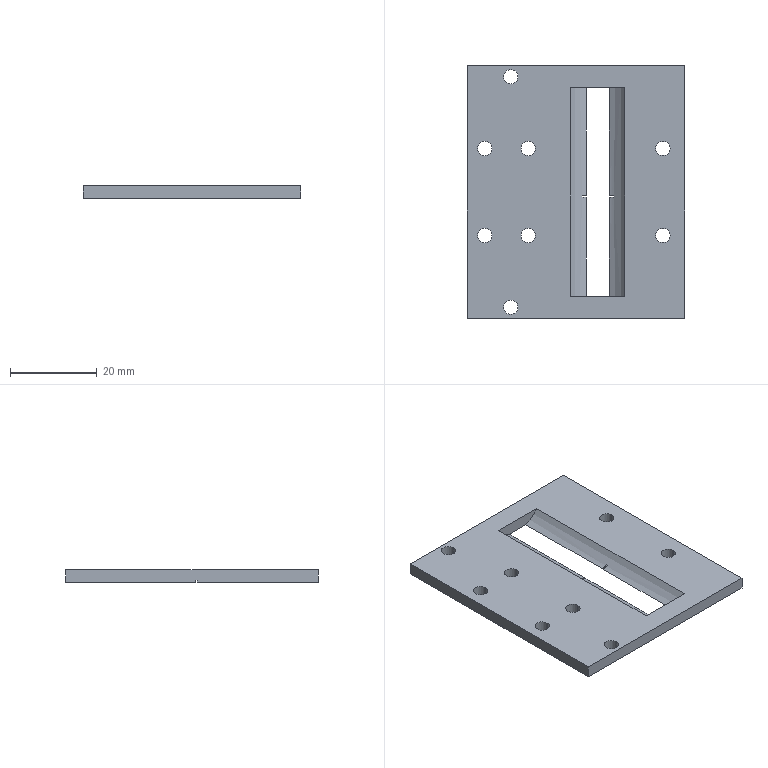Part | SolidWorks | features ICE 3, Extrusion 1 | 1 solid | 33 faces | box 50 x 58 x 2.8 mm | volume 6623 mm3 | cylinder 18 | plane 15 | commonest cylinder face diameters 3.3 x16 15 x2
STEP:
#1=CARTESIAN_POINT('',(-30.658,18.937,0.));
#2=VERTEX_POINT('',#1);
#3=CARTESIAN_POINT('',(-27.358,18.937,0.));
#4=VERTEX_POINT('',#3);
#5=CARTESIAN_POINT('',(-29.008,18.937,0.));
#6=DIRECTION('',(0.,0.,1.));
#7=DIRECTION('',(1.,0.,0.));
#8=AXIS2_PLACEMENT_3D('',#5,#6,#7);
#9=CIRCLE('',#8,1.65);
#10=EDGE_CURVE('',#2,#4,#9,.T.);
#11=ORIENTED_EDGE('',*,*,#10,.F.);
#12=CARTESIAN_POINT('',(-30.658,18.937,2.8));
#13=VERTEX_POINT('',#12);
#14=CARTESIAN_POINT('',(-30.658,18.937,0.));
#15=DIRECTION('',(0.,0.,1.));
#16=VECTOR('',#15,1000.);
#17=LINE('',#14,#16);
#18=EDGE_CURVE('',#2,#13,#17,.T.);
#19=ORIENTED_EDGE('',*,*,#18,.T.);
#20=CARTESIAN_POINT('',(-27.358,18.937,2.8));
#21=VERTEX_POINT('',#20);
#22=CARTESIAN_POINT('',(-29.008,18.937,2.8));
#23=DIRECTION('',(0.,0.,1.));
#24=DIRECTION('',(1.,0.,0.));
#25=AXIS2_PLACEMENT_3D('',#22,#23,#24);
#26=CIRCLE('',#25,1.65);
#27=EDGE_CURVE('',#13,#21,#26,.T.);
#28=ORIENTED_EDGE('',*,*,#27,.T.);
#29=CARTESIAN_POINT('',(-27.358,18.937,0.));
#30=DIRECTION('',(0.,0.,1.));
#31=VECTOR('',#30,1000.);
#32=LINE('',#29,#31);
#33=EDGE_CURVE('',#4,#21,#32,.T.);
#34=ORIENTED_EDGE('',*,*,#33,.F.);
#35=EDGE_LOOP('',(#11,#19,#28,#34));
#36=FACE_OUTER_BOUND('',#35,.T.);
#37=CARTESIAN_POINT('',(-29.008,18.937,0.));
#38=DIRECTION('',(0.,0.,1.));
#39=DIRECTION('',(1.,0.,0.));
#40=AXIS2_PLACEMENT_3D('',#37,#38,#39);
#41=CYLINDRICAL_SURFACE('',#40,1.65);
#42=ADVANCED_FACE('',(#36),#41,.F.);
#43=CARTESIAN_POINT('',(4.342,-17.563,0.));
#44=VERTEX_POINT('',#43);
#45=CARTESIAN_POINT('',(7.642,-17.563,0.));
#46=VERTEX_POINT('',#45);
#47=CARTESIAN_POINT('',(5.992,-17.563,0.));
#48=DIRECTION('',(0.,0.,1.));
#49=DIRECTION('',(1.,0.,0.));
#50=AXIS2_PLACEMENT_3D('',#47,#48,#49);
#51=CIRCLE('',#50,1.65);
#52=EDGE_CURVE('',#44,#46,#51,.T.);
#53=ORIENTED_EDGE('',*,*,#52,.F.);
#54=CARTESIAN_POINT('',(4.342,-17.563,2.8));
#55=VERTEX_POINT('',#54);
#56=CARTESIAN_POINT('',(4.342,-17.563,0.));
#57=DIRECTION('',(0.,0.,1.));
#58=VECTOR('',#57,1000.);
#59=LINE('',#56,#58);
#60=EDGE_CURVE('',#44,#55,#59,.T.);
#61=ORIENTED_EDGE('',*,*,#60,.T.);
#62=CARTESIAN_POINT('',(7.642,-17.563,2.8));
#63=VERTEX_POINT('',#62);
#64=CARTESIAN_POINT('',(5.992,-17.563,2.8));
#65=DIRECTION('',(0.,0.,1.));
#66=DIRECTION('',(1.,0.,0.));
#67=AXIS2_PLACEMENT_3D('',#64,#65,#66);
#68=CIRCLE('',#67,1.65);
#69=EDGE_CURVE('',#55,#63,#68,.T.);
#70=ORIENTED_EDGE('',*,*,#69,.T.);
#71=CARTESIAN_POINT('',(7.642,-17.563,0.));
#72=DIRECTION('',(0.,0.,1.));
#73=VECTOR('',#72,1000.);
#74=LINE('',#71,#73);
#75=EDGE_CURVE('',#46,#63,#74,.T.);
#76=ORIENTED_EDGE('',*,*,#75,.F.);
#77=EDGE_LOOP('',(#53,#61,#70,#76));
#78=FACE_OUTER_BOUND('',#77,.T.);
#79=CARTESIAN_POINT('',(5.992,-17.563,0.));
#80=DIRECTION('',(0.,0.,1.));
#81=DIRECTION('',(1.,0.,0.));
#82=AXIS2_PLACEMENT_3D('',#79,#80,#81);
#83=CYLINDRICAL_SURFACE('',#82,1.65);
#84=ADVANCED_FACE('',(#78),#83,.F.);
#85=CARTESIAN_POINT('',(-30.658,-34.063,0.));
#86=VERTEX_POINT('',#85);
#87=CARTESIAN_POINT('',(-27.358,-34.063,0.));
#88=VERTEX_POINT('',#87);
#89=CARTESIAN_POINT('',(-29.008,-34.063,0.));
#90=DIRECTION('',(0.,0.,1.));
#91=DIRECTION('',(1.,0.,0.));
#92=AXIS2_PLACEMENT_3D('',#89,#90,#91);
#93=CIRCLE('',#92,1.65);
#94=EDGE_CURVE('',#86,#88,#93,.T.);
#95=ORIENTED_EDGE('',*,*,#94,.F.);
#96=CARTESIAN_POINT('',(-30.658,-34.063,2.8));
#97=VERTEX_POINT('',#96);
#98=CARTESIAN_POINT('',(-30.658,-34.063,0.));
#99=DIRECTION('',(0.,0.,1.));
#100=VECTOR('',#99,1000.);
#101=LINE('',#98,#100);
#102=EDGE_CURVE('',#86,#97,#101,.T.);
#103=ORIENTED_EDGE('',*,*,#102,.T.);
#104=CARTESIAN_POINT('',(-27.358,-34.063,2.8));
#105=VERTEX_POINT('',#104);
#106=CARTESIAN_POINT('',(-29.008,-34.063,2.8));
#107=DIRECTION('',(0.,0.,1.));
#108=DIRECTION('',(1.,0.,0.));
#109=AXIS2_PLACEMENT_3D('',#106,#107,#108);
#110=CIRCLE('',#109,1.65);
#111=EDGE_CURVE('',#97,#105,#110,.T.);
#112=ORIENTED_EDGE('',*,*,#111,.T.);
#113=CARTESIAN_POINT('',(-27.358,-34.063,0.));
#114=DIRECTION('',(0.,0.,1.));
#115=VECTOR('',#114,1000.);
#116=LINE('',#113,#115);
#117=EDGE_CURVE('',#88,#105,#116,.T.);
#118=ORIENTED_EDGE('',*,*,#117,.F.);
#119=EDGE_LOOP('',(#95,#103,#112,#118));
#120=FACE_OUTER_BOUND('',#119,.T.);
#121=CARTESIAN_POINT('',(-29.008,-34.063,0.));
#122=DIRECTION('',(0.,0.,1.));
#123=DIRECTION('',(1.,0.,0.));
#124=AXIS2_PLACEMENT_3D('',#121,#122,#123);
#125=CYLINDRICAL_SURFACE('',#124,1.65);
#126=ADVANCED_FACE('',(#120),#125,.F.);
#127=CARTESIAN_POINT('',(-26.658,-17.563,0.));
#128=VERTEX_POINT('',#127);
#129=CARTESIAN_POINT('',(-23.358,-17.563,0.));
#130=VERTEX_POINT('',#129);
#131=CARTESIAN_POINT('',(-25.008,-17.563,0.));
#132=DIRECTION('',(0.,0.,1.));
#133=DIRECTION('',(1.,0.,0.));
#134=AXIS2_PLACEMENT_3D('',#131,#132,#133);
#135=CIRCLE('',#134,1.65);
#136=EDGE_CURVE('',#128,#130,#135,.T.);
#137=ORIENTED_EDGE('',*,*,#136,.F.);
#138=CARTESIAN_POINT('',(-26.658,-17.563,2.8));
#139=VERTEX_POINT('',#138);
#140=CARTESIAN_POINT('',(-26.658,-17.563,0.));
#141=DIRECTION('',(0.,0.,1.));
#142=VECTOR('',#141,1000.);
#143=LINE('',#140,#142);
#144=EDGE_CURVE('',#128,#139,#143,.T.);
#145=ORIENTED_EDGE('',*,*,#144,.T.);
#146=CARTESIAN_POINT('',(-23.358,-17.563,2.8));
#147=VERTEX_POINT('',#146);
#148=CARTESIAN_POINT('',(-25.008,-17.563,2.8));
#149=DIRECTION('',(0.,0.,1.));
#150=DIRECTION('',(1.,0.,0.));
#151=AXIS2_PLACEMENT_3D('',#148,#149,#150);
#152=CIRCLE('',#151,1.65);
#153=EDGE_CURVE('',#139,#147,#152,.T.);
#154=ORIENTED_EDGE('',*,*,#153,.T.);
#155=CARTESIAN_POINT('',(-23.358,-17.563,0.));
#156=DIRECTION('',(0.,0.,1.));
#157=VECTOR('',#156,1000.);
#158=LINE('',#155,#157);
#159=EDGE_CURVE('',#130,#147,#158,.T.);
#160=ORIENTED_EDGE('',*,*,#159,.F.);
#161=EDGE_LOOP('',(#137,#145,#154,#160));
#162=FACE_OUTER_BOUND('',#161,.T.);
#163=CARTESIAN_POINT('',(-25.008,-17.563,0.));
#164=DIRECTION('',(0.,0.,1.));
#165=DIRECTION('',(1.,0.,0.));
#166=AXIS2_PLACEMENT_3D('',#163,#164,#165);
#167=CYLINDRICAL_SURFACE('',#166,1.65);
#168=ADVANCED_FACE('',(#162),#167,.F.);
#169=CARTESIAN_POINT('',(-36.658,2.437,0.));
#170=VERTEX_POINT('',#169);
#171=CARTESIAN_POINT('',(-33.358,2.437,0.));
#172=VERTEX_POINT('',#171);
#173=CARTESIAN_POINT('',(-35.008,2.437,0.));
#174=DIRECTION('',(0.,0.,1.));
#175=DIRECTION('',(1.,0.,0.));
#176=AXIS2_PLACEMENT_3D('',#173,#174,#175);
#177=CIRCLE('',#176,1.65);
#178=EDGE_CURVE('',#170,#172,#177,.T.);
#179=ORIENTED_EDGE('',*,*,#178,.F.);
#180=CARTESIAN_POINT('',(-36.658,2.437,2.8));
#181=VERTEX_POINT('',#180);
#182=CARTESIAN_POINT('',(-36.658,2.437,0.));
#183=DIRECTION('',(0.,0.,1.));
#184=VECTOR('',#183,1000.);
#185=LINE('',#182,#184);
#186=EDGE_CURVE('',#170,#181,#185,.T.);
#187=ORIENTED_EDGE('',*,*,#186,.T.);
#188=CARTESIAN_POINT('',(-33.358,2.437,2.8));
#189=VERTEX_POINT('',#188);
#190=CARTESIAN_POINT('',(-35.008,2.437,2.8));
#191=DIRECTION('',(0.,0.,1.));
#192=DIRECTION('',(1.,0.,0.));
#193=AXIS2_PLACEMENT_3D('',#190,#191,#192);
#194=CIRCLE('',#193,1.65);
#195=EDGE_CURVE('',#181,#189,#194,.T.);
#196=ORIENTED_EDGE('',*,*,#195,.T.);
#197=CARTESIAN_POINT('',(-33.358,2.437,0.));
#198=DIRECTION('',(0.,0.,1.));
#199=VECTOR('',#198,1000.);
#200=LINE('',#197,#199);
#201=EDGE_CURVE('',#172,#189,#200,.T.);
#202=ORIENTED_EDGE('',*,*,#201,.F.);
#203=EDGE_LOOP('',(#179,#187,#196,#202));
#204=FACE_OUTER_BOUND('',#203,.T.);
#205=CARTESIAN_POINT('',(-35.008,2.437,0.));
#206=DIRECTION('',(0.,0.,1.));
#207=DIRECTION('',(1.,0.,0.));
#208=AXIS2_PLACEMENT_3D('',#205,#206,#207);
#209=CYLINDRICAL_SURFACE('',#208,1.65);
#210=ADVANCED_FACE('',(#204),#209,.F.);
#211=CARTESIAN_POINT('',(-26.658,2.437,0.));
#212=VERTEX_POINT('',#211);
#213=CARTESIAN_POINT('',(-23.358,2.437,0.));
#214=VERTEX_POINT('',#213);
#215=CARTESIAN_POINT('',(-25.008,2.437,0.));
#216=DIRECTION('',(0.,0.,1.));
#217=DIRECTION('',(1.,0.,0.));
#218=AXIS2_PLACEMENT_3D('',#215,#216,#217);
#219=CIRCLE('',#218,1.65);
#220=EDGE_CURVE('',#212,#214,#219,.T.);
#221=ORIENTED_EDGE('',*,*,#220,.F.);
#222=CARTESIAN_POINT('',(-26.658,2.437,2.8));
#223=VERTEX_POINT('',#222);
#224=CARTESIAN_POINT('',(-26.658,2.437,0.));
#225=DIRECTION('',(0.,0.,1.));
#226=VECTOR('',#225,1000.);
#227=LINE('',#224,#226);
#228=EDGE_CURVE('',#212,#223,#227,.T.);
#229=ORIENTED_EDGE('',*,*,#228,.T.);
#230=CARTESIAN_POINT('',(-23.358,2.437,2.8));
#231=VERTEX_POINT('',#230);
#232=CARTESIAN_POINT('',(-25.008,2.437,2.8));
#233=DIRECTION('',(0.,0.,1.));
#234=DIRECTION('',(1.,0.,0.));
#235=AXIS2_PLACEMENT_3D('',#232,#233,#234);
#236=CIRCLE('',#235,1.65);
#237=EDGE_CURVE('',#223,#231,#236,.T.);
#238=ORIENTED_EDGE('',*,*,#237,.T.);
#239=CARTESIAN_POINT('',(-23.358,2.437,0.));
#240=DIRECTION('',(0.,0.,1.));
#241=VECTOR('',#240,1000.);
#242=LINE('',#239,#241);
#243=EDGE_CURVE('',#214,#231,#242,.T.);
#244=ORIENTED_EDGE('',*,*,#243,.F.);
#245=EDGE_LOOP('',(#221,#229,#238,#244));
#246=FACE_OUTER_BOUND('',#245,.T.);
#247=CARTESIAN_POINT('',(-25.008,2.437,0.));
#248=DIRECTION('',(0.,0.,1.));
#249=DIRECTION('',(1.,0.,0.));
#250=AXIS2_PLACEMENT_3D('',#247,#248,#249);
#251=CYLINDRICAL_SURFACE('',#250,1.65);
#252=ADVANCED_FACE('',(#246),#251,.F.);
#253=CARTESIAN_POINT('',(4.342,2.437,0.));
#254=VERTEX_POINT('',#253);
#255=CARTESIAN_POINT('',(7.642,2.437,0.));
#256=VERTEX_POINT('',#255);
#257=CARTESIAN_POINT('',(5.992,2.437,0.));
#258=DIRECTION('',(0.,0.,1.));
#259=DIRECTION('',(1.,0.,0.));
#260=AXIS2_PLACEMENT_3D('',#257,#258,#259);
#261=CIRCLE('',#260,1.65);
#262=EDGE_CURVE('',#254,#256,#261,.T.);
#263=ORIENTED_EDGE('',*,*,#262,.F.);
#264=CARTESIAN_POINT('',(4.342,2.437,2.8));
#265=VERTEX_POINT('',#264);
#266=CARTESIAN_POINT('',(4.342,2.437,0.));
#267=DIRECTION('',(0.,0.,1.));
#268=VECTOR('',#267,1000.);
#269=LINE('',#266,#268);
#270=EDGE_CURVE('',#254,#265,#269,.T.);
#271=ORIENTED_EDGE('',*,*,#270,.T.);
#272=CARTESIAN_POINT('',(7.642,2.437,2.8));
#273=VERTEX_POINT('',#272);
#274=CARTESIAN_POINT('',(5.992,2.437,2.8));
#275=DIRECTION('',(0.,0.,1.));
#276=DIRECTION('',(1.,0.,0.));
#277=AXIS2_PLACEMENT_3D('',#274,#275,#276);
#278=CIRCLE('',#277,1.65);
#279=EDGE_CURVE('',#265,#273,#278,.T.);
#280=ORIENTED_EDGE('',*,*,#279,.T.);
#281=CARTESIAN_POINT('',(7.642,2.437,0.));
#282=DIRECTION('',(0.,0.,1.));
#283=VECTOR('',#282,1000.);
#284=LINE('',#281,#283);
#285=EDGE_CURVE('',#256,#273,#284,.T.);
#286=ORIENTED_EDGE('',*,*,#285,.F.);
#287=EDGE_LOOP('',(#263,#271,#280,#286));
#288=FACE_OUTER_BOUND('',#287,.T.);
#289=CARTESIAN_POINT('',(5.992,2.437,0.));
#290=DIRECTION('',(0.,0.,1.));
#291=DIRECTION('',(1.,0.,0.));
#292=AXIS2_PLACEMENT_3D('',#289,#290,#291);
#293=CYLINDRICAL_SURFACE('',#292,1.65);
#294=ADVANCED_FACE('',(#288),#293,.F.);
#295=CARTESIAN_POINT('',(-36.658,-17.563,0.));
#296=VERTEX_POINT('',#295);
#297=CARTESIAN_POINT('',(-33.358,-17.563,0.));
#298=VERTEX_POINT('',#297);
#299=CARTESIAN_POINT('',(-35.008,-17.563,0.));
#300=DIRECTION('',(0.,0.,1.));
#301=DIRECTION('',(1.,0.,0.));
#302=AXIS2_PLACEMENT_3D('',#299,#300,#301);
#303=CIRCLE('',#302,1.65);
#304=EDGE_CURVE('',#296,#298,#303,.T.);
#305=ORIENTED_EDGE('',*,*,#304,.F.);
#306=CARTESIAN_POINT('',(-36.658,-17.563,2.8));
#307=VERTEX_POINT('',#306);
#308=CARTESIAN_POINT('',(-36.658,-17.563,0.));
#309=DIRECTION('',(0.,0.,1.));
#310=VECTOR('',#309,1000.);
#311=LINE('',#308,#310);
#312=EDGE_CURVE('',#296,#307,#311,.T.);
#313=ORIENTED_EDGE('',*,*,#312,.T.);
#314=CARTESIAN_POINT('',(-33.358,-17.563,2.8));
#315=VERTEX_POINT('',#314);
#316=CARTESIAN_POINT('',(-35.008,-17.563,2.8));
#317=DIRECTION('',(0.,0.,1.));
#318=DIRECTION('',(1.,0.,0.));
#319=AXIS2_PLACEMENT_3D('',#316,#317,#318);
#320=CIRCLE('',#319,1.65);
#321=EDGE_CURVE('',#307,#315,#320,.T.);
#322=ORIENTED_EDGE('',*,*,#321,.T.);
#323=CARTESIAN_POINT('',(-33.358,-17.563,0.));
#324=DIRECTION('',(0.,0.,1.));
#325=VECTOR('',#324,1000.);
#326=LINE('',#323,#325);
#327=EDGE_CURVE('',#298,#315,#326,.T.);
#328=ORIENTED_EDGE('',*,*,#327,.F.);
#329=EDGE_LOOP('',(#305,#313,#322,#328));
#330=FACE_OUTER_BOUND('',#329,.T.);
#331=CARTESIAN_POINT('',(-35.008,-17.563,0.));
#332=DIRECTION('',(0.,0.,1.));
#333=DIRECTION('',(1.,0.,0.));
#334=AXIS2_PLACEMENT_3D('',#331,#332,#333);
#335=CYLINDRICAL_SURFACE('',#334,1.65);
#336=ADVANCED_FACE('',(#330),#335,.F.);
#337=CARTESIAN_POINT('',(-29.008,18.937,2.8));
#338=DIRECTION('',(0.,0.,1.));
#339=DIRECTION('',(1.,0.,0.));
#340=AXIS2_PLACEMENT_3D('',#337,#338,#339);
#341=CIRCLE('',#340,1.65);
#342=EDGE_CURVE('',#21,#13,#341,.T.);
#343=ORIENTED_EDGE('',*,*,#342,.F.);
#344=ORIENTED_EDGE('',*,*,#27,.F.);
#345=EDGE_LOOP('',(#343,#344));
#346=FACE_BOUND('',#345,.T.);
#347=CARTESIAN_POINT('',(5.992,-17.563,2.8));
#348=DIRECTION('',(0.,0.,1.));
#349=DIRECTION('',(1.,0.,0.));
#350=AXIS2_PLACEMENT_3D('',#347,#348,#349);
#351=CIRCLE('',#350,1.65);
#352=EDGE_CURVE('',#63,#55,#351,.T.);
#353=ORIENTED_EDGE('',*,*,#352,.F.);
#354=ORIENTED_EDGE('',*,*,#69,.F.);
#355=EDGE_LOOP('',(#353,#354));
#356=FACE_BOUND('',#355,.T.);
#357=CARTESIAN_POINT('',(-29.008,-34.063,2.8));
#358=DIRECTION('',(0.,0.,1.));
#359=DIRECTION('',(1.,0.,0.));
#360=AXIS2_PLACEMENT_3D('',#357,#358,#359);
#361=CIRCLE('',#360,1.65);
#362=EDGE_CURVE('',#105,#97,#361,.T.);
#363=ORIENTED_EDGE('',*,*,#362,.F.);
#364=ORIENTED_EDGE('',*,*,#111,.F.);
#365=EDGE_LOOP('',(#363,#364));
#366=FACE_BOUND('',#365,.T.);
#367=CARTESIAN_POINT('',(-25.008,-17.563,2.8));
#368=DIRECTION('',(0.,0.,1.));
#369=DIRECTION('',(1.,0.,0.));
#370=AXIS2_PLACEMENT_3D('',#367,#368,#369);
#371=CIRCLE('',#370,1.65);
#372=EDGE_CURVE('',#147,#139,#371,.T.);
#373=ORIENTED_EDGE('',*,*,#372,.F.);
#374=ORIENTED_EDGE('',*,*,#153,.F.);
#375=EDGE_LOOP('',(#373,#374));
#376=FACE_BOUND('',#375,.T.);
#377=CARTESIAN_POINT('',(-35.008,2.437,2.8));
#378=DIRECTION('',(0.,0.,1.));
#379=DIRECTION('',(1.,0.,0.));
#380=AXIS2_PLACEMENT_3D('',#377,#378,#379);
#381=CIRCLE('',#380,1.65);
#382=EDGE_CURVE('',#189,#181,#381,.T.);
#383=ORIENTED_EDGE('',*,*,#382,.F.);
#384=ORIENTED_EDGE('',*,*,#195,.F.);
#385=EDGE_LOOP('',(#383,#384));
#386=FACE_BOUND('',#385,.T.);
#387=CARTESIAN_POINT('',(-25.008,2.437,2.8));
#388=DIRECTION('',(0.,0.,1.));
#389=DIRECTION('',(1.,0.,0.));
#390=AXIS2_PLACEMENT_3D('',#387,#388,#389);
#391=CIRCLE('',#390,1.65);
#392=EDGE_CURVE('',#231,#223,#391,.T.);
#393=ORIENTED_EDGE('',*,*,#392,.F.);
#394=ORIENTED_EDGE('',*,*,#237,.F.);
#395=EDGE_LOOP('',(#393,#394));
#396=FACE_BOUND('',#395,.T.);
#397=CARTESIAN_POINT('',(5.992,2.437,2.8));
#398=DIRECTION('',(0.,0.,1.));
#399=DIRECTION('',(1.,0.,0.));
#400=AXIS2_PLACEMENT_3D('',#397,#398,#399);
#401=CIRCLE('',#400,1.65);
#402=EDGE_CURVE('',#273,#265,#401,.T.);
#403=ORIENTED_EDGE('',*,*,#402,.F.);
#404=ORIENTED_EDGE('',*,*,#279,.F.);
#405=EDGE_LOOP('',(#403,#404));
#406=FACE_BOUND('',#405,.T.);
#407=CARTESIAN_POINT('',(-35.008,-17.563,2.8));
#408=DIRECTION('',(0.,0.,1.));
#409=DIRECTION('',(1.,0.,0.));
#410=AXIS2_PLACEMENT_3D('',#407,#408,#409);
#411=CIRCLE('',#410,1.65);
#412=EDGE_CURVE('',#315,#307,#411,.T.);
#413=ORIENTED_EDGE('',*,*,#412,.F.);
#414=ORIENTED_EDGE('',*,*,#321,.F.);
#415=EDGE_LOOP('',(#413,#414));
#416=FACE_BOUND('',#415,.T.);
#417=CARTESIAN_POINT('',(-39.008,21.437,2.8));
#418=VERTEX_POINT('',#417);
#419=CARTESIAN_POINT('',(-39.008,-36.563,2.8));
#420=VERTEX_POINT('',#419);
#421=CARTESIAN_POINT('',(-39.008,21.437,2.8));
#422=DIRECTION('',(0.,-1.,0.));
#423=VECTOR('',#422,1000.);
#424=LINE('',#421,#423);
#425=EDGE_CURVE('',#418,#420,#424,.T.);
#426=ORIENTED_EDGE('',*,*,#425,.T.);
#427=CARTESIAN_POINT('',(10.992,-36.563,2.8));
#428=VERTEX_POINT('',#427);
#429=CARTESIAN_POINT('',(-39.008,-36.563,2.8));
#430=DIRECTION('',(1.,0.,0.));
#431=VECTOR('',#430,1000.);
#432=LINE('',#429,#431);
#433=EDGE_CURVE('',#420,#428,#432,.T.);
#434=ORIENTED_EDGE('',*,*,#433,.T.);
#435=CARTESIAN_POINT('',(10.992,21.437,2.8));
#436=VERTEX_POINT('',#435);
#437=CARTESIAN_POINT('',(10.992,21.437,2.8));
#438=DIRECTION('',(0.,1.,0.));
#439=VECTOR('',#438,1000.);
#440=LINE('',#437,#439);
#441=EDGE_CURVE('',#428,#436,#440,.T.);
#442=ORIENTED_EDGE('',*,*,#441,.T.);
#443=CARTESIAN_POINT('',(-39.008,21.437,2.8));
#444=DIRECTION('',(-1.,0.,0.));
#445=VECTOR('',#444,1000.);
#446=LINE('',#443,#445);
#447=EDGE_CURVE('',#436,#418,#446,.T.);
#448=ORIENTED_EDGE('',*,*,#447,.T.);
#449=EDGE_LOOP('',(#426,#434,#442,#448));
#450=FACE_OUTER_BOUND('',#449,.T.);
#451=CARTESIAN_POINT('',(-2.794,-31.563,2.8));
#452=VERTEX_POINT('',#451);
#453=CARTESIAN_POINT('',(-2.794,16.437,2.8));
#454=VERTEX_POINT('',#453);
#455=CARTESIAN_POINT('',(-2.794,-31.563,2.8));
#456=DIRECTION('',(0.,1.,0.));
#457=VECTOR('',#456,1000.);
#458=LINE('',#455,#457);
#459=EDGE_CURVE('',#452,#454,#458,.T.);
#460=ORIENTED_EDGE('',*,*,#459,.F.);
#461=CARTESIAN_POINT('',(-15.222,-31.563,2.8));
#462=VERTEX_POINT('',#461);
#463=CARTESIAN_POINT('',(-2.794,-31.563,2.8));
#464=DIRECTION('',(1.,0.,0.));
#465=VECTOR('',#464,1000.);
#466=LINE('',#463,#465);
#467=EDGE_CURVE('',#462,#452,#466,.T.);
#468=ORIENTED_EDGE('',*,*,#467,.F.);
#469=CARTESIAN_POINT('',(-15.222,16.437,2.8));
#470=VERTEX_POINT('',#469);
#471=CARTESIAN_POINT('',(-15.222,-31.563,2.8));
#472=DIRECTION('',(0.,1.,0.));
#473=VECTOR('',#472,1000.);
#474=LINE('',#471,#473);
#475=EDGE_CURVE('',#462,#470,#474,.T.);
#476=ORIENTED_EDGE('',*,*,#475,.T.);
#477=CARTESIAN_POINT('',(-2.794,16.437,2.8));
#478=DIRECTION('',(1.,0.,0.));
#479=VECTOR('',#478,1000.);
#480=LINE('',#477,#479);
#481=EDGE_CURVE('',#470,#454,#480,.T.);
#482=ORIENTED_EDGE('',*,*,#481,.T.);
#483=EDGE_LOOP('',(#460,#468,#476,#482));
#484=FACE_BOUND('',#483,.T.);
#485=CARTESIAN_POINT('',(0.,0.,2.8));
#486=DIRECTION('',(0.,0.,1.));
#487=DIRECTION('',(1.,0.,0.));
#488=AXIS2_PLACEMENT_3D('',#485,#486,#487);
#489=PLANE('',#488);
#490=ADVANCED_FACE('',(#346,#356,#366,#376,#386,#396,#406,#416,#450,#484),#489,.T.);
#491=CARTESIAN_POINT('',(-6.315,-8.813,0.));
#492=VERTEX_POINT('',#491);
#493=CARTESIAN_POINT('',(10.992,-8.813,0.));
#494=VERTEX_POINT('',#493);
#495=CARTESIAN_POINT('',(-39.008,-8.813,0.));
#496=DIRECTION('',(1.,0.,0.));
#497=VECTOR('',#496,1000.);
#498=LINE('',#495,#497);
#499=EDGE_CURVE('',#492,#494,#498,.T.);
#500=ORIENTED_EDGE('',*,*,#499,.F.);
#501=CARTESIAN_POINT('',(-5.354,-8.813,0.45));
#502=VERTEX_POINT('',#501);
#503=CARTESIAN_POINT('',(-9.008,-8.813,7.));
#504=DIRECTION('',(0.,-1.,0.));
#505=DIRECTION('',(1.,0.,0.));
#506=AXIS2_PLACEMENT_3D('',#503,#504,#505);
#507=CIRCLE('',#506,7.5);
#508=EDGE_CURVE('',#492,#502,#507,.T.);
#509=ORIENTED_EDGE('',*,*,#508,.T.);
#510=CARTESIAN_POINT('',(10.992,-8.813,0.45));
#511=VERTEX_POINT('',#510);
#512=CARTESIAN_POINT('',(-39.008,-8.813,0.45));
#513=DIRECTION('',(1.,0.,0.));
#514=VECTOR('',#513,1000.);
#515=LINE('',#512,#514);
#516=EDGE_CURVE('',#502,#511,#515,.T.);
#517=ORIENTED_EDGE('',*,*,#516,.T.);
#518=CARTESIAN_POINT('',(10.992,-8.813,0.));
#519=DIRECTION('',(0.,0.,-1.));
#520=VECTOR('',#519,1000.);
#521=LINE('',#518,#520);
#522=EDGE_CURVE('',#511,#494,#521,.T.);
#523=ORIENTED_EDGE('',*,*,#522,.T.);
#524=EDGE_LOOP('',(#500,#509,#517,#523));
#525=FACE_OUTER_BOUND('',#524,.T.);
#526=CARTESIAN_POINT('',(-39.008,-8.813,0.));
#527=DIRECTION('',(0.,-1.,0.));
#528=DIRECTION('',(1.,0.,0.));
#529=AXIS2_PLACEMENT_3D('',#526,#527,#528);
#530=PLANE('',#529);
#531=ADVANCED_FACE('',(#525),#530,.F.);
#532=ORIENTED_EDGE('',*,*,#516,.F.);
#533=CARTESIAN_POINT('',(-5.354,-8.363,0.45));
#534=VERTEX_POINT('',#533);
#535=CARTESIAN_POINT('',(-5.354,-31.563,0.45));
#536=DIRECTION('',(0.,1.,0.));
#537=VECTOR('',#536,1000.);
#538=LINE('',#535,#537);
#539=EDGE_CURVE('',#502,#534,#538,.T.);
#540=ORIENTED_EDGE('',*,*,#539,.T.);
#541=CARTESIAN_POINT('',(10.992,-8.363,0.45));
#542=VERTEX_POINT('',#541);
#543=CARTESIAN_POINT('',(-39.008,-8.363,0.45));
#544=DIRECTION('',(1.,0.,0.));
#545=VECTOR('',#544,1000.);
#546=LINE('',#543,#545);
#547=EDGE_CURVE('',#534,#542,#546,.T.);
#548=ORIENTED_EDGE('',*,*,#547,.T.);
#549=CARTESIAN_POINT('',(10.992,-8.813,0.45));
#550=DIRECTION('',(0.,-1.,0.));
#551=VECTOR('',#550,1000.);
#552=LINE('',#549,#551);
#553=EDGE_CURVE('',#542,#511,#552,.T.);
#554=ORIENTED_EDGE('',*,*,#553,.T.);
#555=EDGE_LOOP('',(#532,#540,#548,#554));
#556=FACE_OUTER_BOUND('',#555,.T.);
#557=CARTESIAN_POINT('',(-39.008,-8.813,0.45));
#558=DIRECTION('',(0.,0.,1.));
#559=DIRECTION('',(1.,0.,0.));
#560=AXIS2_PLACEMENT_3D('',#557,#558,#559);
#561=PLANE('',#560);
#562=ADVANCED_FACE('',(#556),#561,.F.);
#563=ORIENTED_EDGE('',*,*,#547,.F.);
#564=CARTESIAN_POINT('',(-6.315,-8.363,0.));
#565=VERTEX_POINT('',#564);
#566=CARTESIAN_POINT('',(-9.008,-8.363,7.));
#567=DIRECTION('',(0.,1.,0.));
#568=DIRECTION('',(0.,0.,1.));
#569=AXIS2_PLACEMENT_3D('',#566,#567,#568);
#570=CIRCLE('',#569,7.5);
#571=EDGE_CURVE('',#534,#565,#570,.T.);
#572=ORIENTED_EDGE('',*,*,#571,.T.);
#573=CARTESIAN_POINT('',(10.992,-8.363,0.));
#574=VERTEX_POINT('',#573);
#575=CARTESIAN_POINT('',(-39.008,-8.363,0.));
#576=DIRECTION('',(1.,0.,0.));
#577=VECTOR('',#576,1000.);
#578=LINE('',#575,#577);
#579=EDGE_CURVE('',#565,#574,#578,.T.);
#580=ORIENTED_EDGE('',*,*,#579,.T.);
#581=CARTESIAN_POINT('',(10.992,-8.363,0.));
#582=DIRECTION('',(0.,0.,1.));
#583=VECTOR('',#582,1000.);
#584=LINE('',#581,#583);
#585=EDGE_CURVE('',#574,#542,#584,.T.);
#586=ORIENTED_EDGE('',*,*,#585,.T.);
#587=EDGE_LOOP('',(#563,#572,#580,#586));
#588=FACE_OUTER_BOUND('',#587,.T.);
#589=CARTESIAN_POINT('',(-39.008,-8.363,0.));
#590=DIRECTION('',(0.,1.,0.));
#591=DIRECTION('',(0.,0.,1.));
#592=AXIS2_PLACEMENT_3D('',#589,#590,#591);
#593=PLANE('',#592);
#594=ADVANCED_FACE('',(#588),#593,.F.);
#595=CARTESIAN_POINT('',(-35.008,-17.563,0.));
#596=DIRECTION('',(0.,0.,1.));
#597=DIRECTION('',(1.,0.,0.));
#598=AXIS2_PLACEMENT_3D('',#595,#596,#597);
#599=CIRCLE('',#598,1.65);
#600=EDGE_CURVE('',#298,#296,#599,.T.);
#601=ORIENTED_EDGE('',*,*,#600,.T.);
#602=ORIENTED_EDGE('',*,*,#304,.T.);
#603=EDGE_LOOP('',(#601,#602));
#604=FACE_BOUND('',#603,.T.);
#605=CARTESIAN_POINT('',(-25.008,-17.563,0.));
#606=DIRECTION('',(0.,0.,1.));
#607=DIRECTION('',(1.,0.,0.));
#608=AXIS2_PLACEMENT_3D('',#605,#606,#607);
#609=CIRCLE('',#608,1.65);
#610=EDGE_CURVE('',#130,#128,#609,.T.);
#611=ORIENTED_EDGE('',*,*,#610,.T.);
#612=ORIENTED_EDGE('',*,*,#136,.T.);
#613=EDGE_LOOP('',(#611,#612));
#614=FACE_BOUND('',#613,.T.);
#615=CARTESIAN_POINT('',(-29.008,-34.063,0.));
#616=DIRECTION('',(0.,0.,1.));
#617=DIRECTION('',(1.,0.,0.));
#618=AXIS2_PLACEMENT_3D('',#615,#616,#617);
#619=CIRCLE('',#618,1.65);
#620=EDGE_CURVE('',#88,#86,#619,.T.);
#621=ORIENTED_EDGE('',*,*,#620,.T.);
#622=ORIENTED_EDGE('',*,*,#94,.T.);
#623=EDGE_LOOP('',(#621,#622));
#624=FACE_BOUND('',#623,.T.);
#625=CARTESIAN_POINT('',(5.992,-17.563,0.));
#626=DIRECTION('',(0.,0.,1.));
#627=DIRECTION('',(1.,0.,0.));
#628=AXIS2_PLACEMENT_3D('',#625,#626,#627);
#629=CIRCLE('',#628,1.65);
#630=EDGE_CURVE('',#46,#44,#629,.T.);
#631=ORIENTED_EDGE('',*,*,#630,.T.);
#632=ORIENTED_EDGE('',*,*,#52,.T.);
#633=EDGE_LOOP('',(#631,#632));
#634=FACE_BOUND('',#633,.T.);
#635=CARTESIAN_POINT('',(-6.315,-31.563,0.));
#636=VERTEX_POINT('',#635);
#637=CARTESIAN_POINT('',(-11.7,-31.563,0.));
#638=VERTEX_POINT('',#637);
#639=CARTESIAN_POINT('',(0.,-31.563,0.));
#640=DIRECTION('',(-1.,0.,0.));
#641=VECTOR('',#640,1000.);
#642=LINE('',#639,#641);
#643=EDGE_CURVE('',#636,#638,#642,.T.);
#644=ORIENTED_EDGE('',*,*,#643,.F.);
#645=CARTESIAN_POINT('',(-6.315,-31.563,0.));
#646=DIRECTION('',(0.,1.,0.));
#647=VECTOR('',#646,1000.);
#648=LINE('',#645,#647);
#649=EDGE_CURVE('',#636,#492,#648,.T.);
#650=ORIENTED_EDGE('',*,*,#649,.T.);
#651=ORIENTED_EDGE('',*,*,#499,.T.);
#652=CARTESIAN_POINT('',(10.992,-36.563,0.));
#653=VERTEX_POINT('',#652);
#654=CARTESIAN_POINT('',(10.992,21.437,0.));
#655=DIRECTION('',(0.,1.,0.));
#656=VECTOR('',#655,1000.);
#657=LINE('',#654,#656);
#658=EDGE_CURVE('',#653,#494,#657,.T.);
#659=ORIENTED_EDGE('',*,*,#658,.F.);
#660=CARTESIAN_POINT('',(-39.008,-36.563,0.));
#661=VERTEX_POINT('',#660);
#662=CARTESIAN_POINT('',(-39.008,-36.563,0.));
#663=DIRECTION('',(1.,0.,0.));
#664=VECTOR('',#663,1000.);
#665=LINE('',#662,#664);
#666=EDGE_CURVE('',#661,#653,#665,.T.);
#667=ORIENTED_EDGE('',*,*,#666,.F.);
#668=CARTESIAN_POINT('',(-39.008,-8.813,0.));
#669=VERTEX_POINT('',#668);
#670=CARTESIAN_POINT('',(-39.008,21.437,0.));
#671=DIRECTION('',(0.,-1.,0.));
#672=VECTOR('',#671,1000.);
#673=LINE('',#670,#672);
#674=EDGE_CURVE('',#669,#661,#673,.T.);
#675=ORIENTED_EDGE('',*,*,#674,.F.);
#676=CARTESIAN_POINT('',(-11.7,-8.813,0.));
#677=VERTEX_POINT('',#676);
#678=CARTESIAN_POINT('',(-39.008,-8.813,0.));
#679=DIRECTION('',(1.,0.,0.));
#680=VECTOR('',#679,1000.);
#681=LINE('',#678,#680);
#682=EDGE_CURVE('',#669,#677,#681,.T.);
#683=ORIENTED_EDGE('',*,*,#682,.T.);
#684=CARTESIAN_POINT('',(-11.7,-31.563,0.));
#685=DIRECTION('',(0.,1.,0.));
#686=VECTOR('',#685,1000.);
#687=LINE('',#684,#686);
#688=EDGE_CURVE('',#638,#677,#687,.T.);
#689=ORIENTED_EDGE('',*,*,#688,.F.);
#690=EDGE_LOOP('',(#644,#650,#651,#659,#667,#675,#683,#689));
#691=FACE_OUTER_BOUND('',#690,.T.);
#692=CARTESIAN_POINT('',(0.,0.,0.));
#693=DIRECTION('',(0.,0.,1.));
#694=DIRECTION('',(1.,0.,0.));
#695=AXIS2_PLACEMENT_3D('',#692,#693,#694);
#696=PLANE('',#695);
#697=ADVANCED_FACE('',(#604,#614,#624,#634,#691),#696,.F.);
#698=CARTESIAN_POINT('',(-39.008,-8.363,0.45));
#699=VERTEX_POINT('',#698);
#700=CARTESIAN_POINT('',(-39.008,-8.813,0.45));
#701=VERTEX_POINT('',#700);
#702=CARTESIAN_POINT('',(-39.008,-8.813,0.45));
#703=DIRECTION('',(0.,-1.,0.));
#704=VECTOR('',#703,1000.);
#705=LINE('',#702,#704);
#706=EDGE_CURVE('',#699,#701,#705,.T.);
#707=ORIENTED_EDGE('',*,*,#706,.T.);
#708=CARTESIAN_POINT('',(-39.008,-8.813,0.));
#709=DIRECTION('',(0.,0.,-1.));
#710=VECTOR('',#709,1000.);
#711=LINE('',#708,#710);
#712=EDGE_CURVE('',#701,#669,#711,.T.);
#713=ORIENTED_EDGE('',*,*,#712,.T.);
#714=ORIENTED_EDGE('',*,*,#674,.T.);
#715=CARTESIAN_POINT('',(-39.008,-36.563,2.8));
#716=DIRECTION('',(0.,0.,-1.));
#717=VECTOR('',#716,1000.);
#718=LINE('',#715,#717);
#719=EDGE_CURVE('',#420,#661,#718,.T.);
#720=ORIENTED_EDGE('',*,*,#719,.F.);
#721=ORIENTED_EDGE('',*,*,#425,.F.);
#722=CARTESIAN_POINT('',(-39.008,21.437,0.));
#723=VERTEX_POINT('',#722);
#724=CARTESIAN_POINT('',(-39.008,21.437,2.8));
#725=DIRECTION('',(0.,0.,-1.));
#726=VECTOR('',#725,1000.);
#727=LINE('',#724,#726);
#728=EDGE_CURVE('',#418,#723,#727,.T.);
#729=ORIENTED_EDGE('',*,*,#728,.T.);
#730=CARTESIAN_POINT('',(-39.008,-8.363,0.));
#731=VERTEX_POINT('',#730);
#732=CARTESIAN_POINT('',(-39.008,21.437,0.));
#733=DIRECTION('',(0.,-1.,0.));
#734=VECTOR('',#733,1000.);
#735=LINE('',#732,#734);
#736=EDGE_CURVE('',#723,#731,#735,.T.);
#737=ORIENTED_EDGE('',*,*,#736,.T.);
#738=CARTESIAN_POINT('',(-39.008,-8.363,0.));
#739=DIRECTION('',(0.,0.,1.));
#740=VECTOR('',#739,1000.);
#741=LINE('',#738,#740);
#742=EDGE_CURVE('',#731,#699,#741,.T.);
#743=ORIENTED_EDGE('',*,*,#742,.T.);
#744=EDGE_LOOP('',(#707,#713,#714,#720,#721,#729,#737,#743));
#745=FACE_OUTER_BOUND('',#744,.T.);
#746=CARTESIAN_POINT('',(-39.008,21.437,2.8));
#747=DIRECTION('',(1.,0.,0.));
#748=DIRECTION('',(0.,0.,-1.));
#749=AXIS2_PLACEMENT_3D('',#746,#747,#748);
#750=PLANE('',#749);
#751=ADVANCED_FACE('',(#745),#750,.F.);
#752=ORIENTED_EDGE('',*,*,#666,.T.);
#753=CARTESIAN_POINT('',(10.992,-36.563,2.8));
#754=DIRECTION('',(0.,0.,-1.));
#755=VECTOR('',#754,1000.);
#756=LINE('',#753,#755);
#757=EDGE_CURVE('',#428,#653,#756,.T.);
#758=ORIENTED_EDGE('',*,*,#757,.F.);
#759=ORIENTED_EDGE('',*,*,#433,.F.);
#760=ORIENTED_EDGE('',*,*,#719,.T.);
#761=EDGE_LOOP('',(#752,#758,#759,#760));
#762=FACE_OUTER_BOUND('',#761,.T.);
#763=CARTESIAN_POINT('',(-39.008,-36.563,2.8));
#764=DIRECTION('',(0.,1.,0.));
#765=DIRECTION('',(-1.,0.,0.));
#766=AXIS2_PLACEMENT_3D('',#763,#764,#765);
#767=PLANE('',#766);
#768=ADVANCED_FACE('',(#762),#767,.F.);
#769=ORIENTED_EDGE('',*,*,#658,.T.);
#770=ORIENTED_EDGE('',*,*,#522,.F.);
#771=ORIENTED_EDGE('',*,*,#553,.F.);
#772=ORIENTED_EDGE('',*,*,#585,.F.);
#773=CARTESIAN_POINT('',(10.992,21.437,0.));
#774=VERTEX_POINT('',#773);
#775=CARTESIAN_POINT('',(10.992,21.437,0.));
#776=DIRECTION('',(0.,1.,0.));
#777=VECTOR('',#776,1000.);
#778=LINE('',#775,#777);
#779=EDGE_CURVE('',#574,#774,#778,.T.);
#780=ORIENTED_EDGE('',*,*,#779,.T.);
#781=CARTESIAN_POINT('',(10.992,21.437,2.8));
#782=DIRECTION('',(0.,0.,-1.));
#783=VECTOR('',#782,1000.);
#784=LINE('',#781,#783);
#785=EDGE_CURVE('',#436,#774,#784,.T.);
#786=ORIENTED_EDGE('',*,*,#785,.F.);
#787=ORIENTED_EDGE('',*,*,#441,.F.);
#788=ORIENTED_EDGE('',*,*,#757,.T.);
#789=EDGE_LOOP('',(#769,#770,#771,#772,#780,#786,#787,#788));
#790=FACE_OUTER_BOUND('',#789,.T.);
#791=CARTESIAN_POINT('',(10.992,21.437,2.8));
#792=DIRECTION('',(-1.,0.,0.));
#793=DIRECTION('',(0.,-1.,0.));
#794=AXIS2_PLACEMENT_3D('',#791,#792,#793);
#795=PLANE('',#794);
#796=ADVANCED_FACE('',(#790),#795,.F.);
#797=CARTESIAN_POINT('',(-39.008,21.437,0.));
#798=DIRECTION('',(-1.,0.,0.));
#799=VECTOR('',#798,1000.);
#800=LINE('',#797,#799);
#801=EDGE_CURVE('',#774,#723,#800,.T.);
#802=ORIENTED_EDGE('',*,*,#801,.T.);
#803=ORIENTED_EDGE('',*,*,#728,.F.);
#804=ORIENTED_EDGE('',*,*,#447,.F.);
#805=ORIENTED_EDGE('',*,*,#785,.T.);
#806=EDGE_LOOP('',(#802,#803,#804,#805));
#807=FACE_OUTER_BOUND('',#806,.T.);
#808=CARTESIAN_POINT('',(-39.008,21.437,2.8));
#809=DIRECTION('',(0.,-1.,0.));
#810=DIRECTION('',(0.,0.,-1.));
#811=AXIS2_PLACEMENT_3D('',#808,#809,#810);
#812=PLANE('',#811);
#813=ADVANCED_FACE('',(#807),#812,.F.);
#814=ORIENTED_EDGE('',*,*,#579,.F.);
#815=CARTESIAN_POINT('',(-6.315,16.437,0.));
#816=VERTEX_POINT('',#815);
#817=CARTESIAN_POINT('',(-6.315,-31.563,0.));
#818=DIRECTION('',(0.,1.,0.));
#819=VECTOR('',#818,1000.);
#820=LINE('',#817,#819);
#821=EDGE_CURVE('',#565,#816,#820,.T.);
#822=ORIENTED_EDGE('',*,*,#821,.T.);
#823=CARTESIAN_POINT('',(-11.7,16.437,0.));
#824=VERTEX_POINT('',#823);
#825=CARTESIAN_POINT('',(0.,16.437,0.));
#826=DIRECTION('',(-1.,0.,0.));
#827=VECTOR('',#826,1000.);
#828=LINE('',#825,#827);
#829=EDGE_CURVE('',#816,#824,#828,.T.);
#830=ORIENTED_EDGE('',*,*,#829,.T.);
#831=CARTESIAN_POINT('',(-11.7,-8.363,0.));
#832=VERTEX_POINT('',#831);
#833=CARTESIAN_POINT('',(-11.7,-31.563,0.));
#834=DIRECTION('',(0.,1.,0.));
#835=VECTOR('',#834,1000.);
#836=LINE('',#833,#835);
#837=EDGE_CURVE('',#832,#824,#836,.T.);
#838=ORIENTED_EDGE('',*,*,#837,.F.);
#839=CARTESIAN_POINT('',(-39.008,-8.363,0.));
#840=DIRECTION('',(1.,0.,0.));
#841=VECTOR('',#840,1000.);
#842=LINE('',#839,#841);
#843=EDGE_CURVE('',#731,#832,#842,.T.);
#844=ORIENTED_EDGE('',*,*,#843,.F.);
#845=ORIENTED_EDGE('',*,*,#736,.F.);
#846=ORIENTED_EDGE('',*,*,#801,.F.);
#847=ORIENTED_EDGE('',*,*,#779,.F.);
#848=EDGE_LOOP('',(#814,#822,#830,#838,#844,#845,#846,#847));
#849=FACE_OUTER_BOUND('',#848,.T.);
#850=CARTESIAN_POINT('',(-29.008,18.937,0.));
#851=DIRECTION('',(0.,0.,1.));
#852=DIRECTION('',(1.,0.,0.));
#853=AXIS2_PLACEMENT_3D('',#850,#851,#852);
#854=CIRCLE('',#853,1.65);
#855=EDGE_CURVE('',#4,#2,#854,.T.);
#856=ORIENTED_EDGE('',*,*,#855,.T.);
#857=ORIENTED_EDGE('',*,*,#10,.T.);
#858=EDGE_LOOP('',(#856,#857));
#859=FACE_BOUND('',#858,.T.);
#860=CARTESIAN_POINT('',(-35.008,2.437,0.));
#861=DIRECTION('',(0.,0.,1.));
#862=DIRECTION('',(1.,0.,0.));
#863=AXIS2_PLACEMENT_3D('',#860,#861,#862);
#864=CIRCLE('',#863,1.65);
#865=EDGE_CURVE('',#172,#170,#864,.T.);
#866=ORIENTED_EDGE('',*,*,#865,.T.);
#867=ORIENTED_EDGE('',*,*,#178,.T.);
#868=EDGE_LOOP('',(#866,#867));
#869=FACE_BOUND('',#868,.T.);
#870=CARTESIAN_POINT('',(-25.008,2.437,0.));
#871=DIRECTION('',(0.,0.,1.));
#872=DIRECTION('',(1.,0.,0.));
#873=AXIS2_PLACEMENT_3D('',#870,#871,#872);
#874=CIRCLE('',#873,1.65);
#875=EDGE_CURVE('',#214,#212,#874,.T.);
#876=ORIENTED_EDGE('',*,*,#875,.T.);
#877=ORIENTED_EDGE('',*,*,#220,.T.);
#878=EDGE_LOOP('',(#876,#877));
#879=FACE_BOUND('',#878,.T.);
#880=CARTESIAN_POINT('',(5.992,2.437,0.));
#881=DIRECTION('',(0.,0.,1.));
#882=DIRECTION('',(1.,0.,0.));
#883=AXIS2_PLACEMENT_3D('',#880,#881,#882);
#884=CIRCLE('',#883,1.65);
#885=EDGE_CURVE('',#256,#254,#884,.T.);
#886=ORIENTED_EDGE('',*,*,#885,.T.);
#887=ORIENTED_EDGE('',*,*,#262,.T.);
#888=EDGE_LOOP('',(#886,#887));
#889=FACE_BOUND('',#888,.T.);
#890=CARTESIAN_POINT('',(0.,0.,0.));
#891=DIRECTION('',(0.,0.,1.));
#892=DIRECTION('',(1.,0.,0.));
#893=AXIS2_PLACEMENT_3D('',#890,#891,#892);
#894=PLANE('',#893);
#895=ADVANCED_FACE('',(#849,#859,#869,#879,#889),#894,.F.);
#896=ORIENTED_EDGE('',*,*,#312,.F.);
#897=ORIENTED_EDGE('',*,*,#600,.F.);
#898=ORIENTED_EDGE('',*,*,#327,.T.);
#899=ORIENTED_EDGE('',*,*,#412,.T.);
#900=EDGE_LOOP('',(#896,#897,#898,#899));
#901=FACE_OUTER_BOUND('',#900,.T.);
#902=CARTESIAN_POINT('',(-35.008,-17.563,0.));
#903=DIRECTION('',(0.,0.,1.));
#904=DIRECTION('',(1.,0.,0.));
#905=AXIS2_PLACEMENT_3D('',#902,#903,#904);
#906=CYLINDRICAL_SURFACE('',#905,1.65);
#907=ADVANCED_FACE('',(#901),#906,.F.);
#908=ORIENTED_EDGE('',*,*,#270,.F.);
#909=ORIENTED_EDGE('',*,*,#885,.F.);
#910=ORIENTED_EDGE('',*,*,#285,.T.);
#911=ORIENTED_EDGE('',*,*,#402,.T.);
#912=EDGE_LOOP('',(#908,#909,#910,#911));
#913=FACE_OUTER_BOUND('',#912,.T.);
#914=CARTESIAN_POINT('',(5.992,2.437,0.));
#915=DIRECTION('',(0.,0.,1.));
#916=DIRECTION('',(1.,0.,0.));
#917=AXIS2_PLACEMENT_3D('',#914,#915,#916);
#918=CYLINDRICAL_SURFACE('',#917,1.65);
#919=ADVANCED_FACE('',(#913),#918,.F.);
#920=ORIENTED_EDGE('',*,*,#228,.F.);
#921=ORIENTED_EDGE('',*,*,#875,.F.);
#922=ORIENTED_EDGE('',*,*,#243,.T.);
#923=ORIENTED_EDGE('',*,*,#392,.T.);
#924=EDGE_LOOP('',(#920,#921,#922,#923));
#925=FACE_OUTER_BOUND('',#924,.T.);
#926=CARTESIAN_POINT('',(-25.008,2.437,0.));
#927=DIRECTION('',(0.,0.,1.));
#928=DIRECTION('',(1.,0.,0.));
#929=AXIS2_PLACEMENT_3D('',#926,#927,#928);
#930=CYLINDRICAL_SURFACE('',#929,1.65);
#931=ADVANCED_FACE('',(#925),#930,.F.);
#932=ORIENTED_EDGE('',*,*,#186,.F.);
#933=ORIENTED_EDGE('',*,*,#865,.F.);
#934=ORIENTED_EDGE('',*,*,#201,.T.);
#935=ORIENTED_EDGE('',*,*,#382,.T.);
#936=EDGE_LOOP('',(#932,#933,#934,#935));
#937=FACE_OUTER_BOUND('',#936,.T.);
#938=CARTESIAN_POINT('',(-35.008,2.437,0.));
#939=DIRECTION('',(0.,0.,1.));
#940=DIRECTION('',(1.,0.,0.));
#941=AXIS2_PLACEMENT_3D('',#938,#939,#940);
#942=CYLINDRICAL_SURFACE('',#941,1.65);
#943=ADVANCED_FACE('',(#937),#942,.F.);
#944=ORIENTED_EDGE('',*,*,#144,.F.);
#945=ORIENTED_EDGE('',*,*,#610,.F.);
#946=ORIENTED_EDGE('',*,*,#159,.T.);
#947=ORIENTED_EDGE('',*,*,#372,.T.);
#948=EDGE_LOOP('',(#944,#945,#946,#947));
#949=FACE_OUTER_BOUND('',#948,.T.);
#950=CARTESIAN_POINT('',(-25.008,-17.563,0.));
#951=DIRECTION('',(0.,0.,1.));
#952=DIRECTION('',(1.,0.,0.));
#953=AXIS2_PLACEMENT_3D('',#950,#951,#952);
#954=CYLINDRICAL_SURFACE('',#953,1.65);
#955=ADVANCED_FACE('',(#949),#954,.F.);
#956=ORIENTED_EDGE('',*,*,#102,.F.);
#957=ORIENTED_EDGE('',*,*,#620,.F.);
#958=ORIENTED_EDGE('',*,*,#117,.T.);
#959=ORIENTED_EDGE('',*,*,#362,.T.);
#960=EDGE_LOOP('',(#956,#957,#958,#959));
#961=FACE_OUTER_BOUND('',#960,.T.);
#962=CARTESIAN_POINT('',(-29.008,-34.063,0.));
#963=DIRECTION('',(0.,0.,1.));
#964=DIRECTION('',(1.,0.,0.));
#965=AXIS2_PLACEMENT_3D('',#962,#963,#964);
#966=CYLINDRICAL_SURFACE('',#965,1.65);
#967=ADVANCED_FACE('',(#961),#966,.F.);
#968=ORIENTED_EDGE('',*,*,#60,.F.);
#969=ORIENTED_EDGE('',*,*,#630,.F.);
#970=ORIENTED_EDGE('',*,*,#75,.T.);
#971=ORIENTED_EDGE('',*,*,#352,.T.);
#972=EDGE_LOOP('',(#968,#969,#970,#971));
#973=FACE_OUTER_BOUND('',#972,.T.);
#974=CARTESIAN_POINT('',(5.992,-17.563,0.));
#975=DIRECTION('',(0.,0.,1.));
#976=DIRECTION('',(1.,0.,0.));
#977=AXIS2_PLACEMENT_3D('',#974,#975,#976);
#978=CYLINDRICAL_SURFACE('',#977,1.65);
#979=ADVANCED_FACE('',(#973),#978,.F.);
#980=ORIENTED_EDGE('',*,*,#18,.F.);
#981=ORIENTED_EDGE('',*,*,#855,.F.);
#982=ORIENTED_EDGE('',*,*,#33,.T.);
#983=ORIENTED_EDGE('',*,*,#342,.T.);
#984=EDGE_LOOP('',(#980,#981,#982,#983));
#985=FACE_OUTER_BOUND('',#984,.T.);
#986=CARTESIAN_POINT('',(-29.008,18.937,0.));
#987=DIRECTION('',(0.,0.,1.));
#988=DIRECTION('',(1.,0.,0.));
#989=AXIS2_PLACEMENT_3D('',#986,#987,#988);
#990=CYLINDRICAL_SURFACE('',#989,1.65);
#991=ADVANCED_FACE('',(#985),#990,.F.);
#992=CARTESIAN_POINT('',(-12.661,-8.813,0.45));
#993=VERTEX_POINT('',#992);
#994=CARTESIAN_POINT('',(-39.008,-8.813,0.45));
#995=DIRECTION('',(1.,0.,0.));
#996=VECTOR('',#995,1000.);
#997=LINE('',#994,#996);
#998=EDGE_CURVE('',#701,#993,#997,.T.);
#999=ORIENTED_EDGE('',*,*,#998,.T.);
#1000=CARTESIAN_POINT('',(-9.008,-8.813,7.));
#1001=DIRECTION('',(0.,-1.,0.));
#1002=DIRECTION('',(1.,0.,0.));
#1003=AXIS2_PLACEMENT_3D('',#1000,#1001,#1002);
#1004=CIRCLE('',#1003,7.5);
#1005=EDGE_CURVE('',#993,#677,#1004,.T.);
#1006=ORIENTED_EDGE('',*,*,#1005,.T.);
#1007=ORIENTED_EDGE('',*,*,#682,.F.);
#1008=ORIENTED_EDGE('',*,*,#712,.F.);
#1009=EDGE_LOOP('',(#999,#1006,#1007,#1008));
#1010=FACE_OUTER_BOUND('',#1009,.T.);
#1011=CARTESIAN_POINT('',(-39.008,-8.813,0.));
#1012=DIRECTION('',(0.,-1.,0.));
#1013=DIRECTION('',(1.,0.,0.));
#1014=AXIS2_PLACEMENT_3D('',#1011,#1012,#1013);
#1015=PLANE('',#1014);
#1016=ADVANCED_FACE('',(#1010),#1015,.F.);
#1017=CARTESIAN_POINT('',(-12.661,-8.363,0.45));
#1018=VERTEX_POINT('',#1017);
#1019=CARTESIAN_POINT('',(-39.008,-8.363,0.45));
#1020=DIRECTION('',(1.,0.,0.));
#1021=VECTOR('',#1020,1000.);
#1022=LINE('',#1019,#1021);
#1023=EDGE_CURVE('',#699,#1018,#1022,.T.);
#1024=ORIENTED_EDGE('',*,*,#1023,.T.);
#1025=CARTESIAN_POINT('',(-12.661,-31.563,0.45));
#1026=DIRECTION('',(0.,-1.,0.));
#1027=VECTOR('',#1026,1000.);
#1028=LINE('',#1025,#1027);
#1029=EDGE_CURVE('',#1018,#993,#1028,.T.);
#1030=ORIENTED_EDGE('',*,*,#1029,.T.);
#1031=ORIENTED_EDGE('',*,*,#998,.F.);
#1032=ORIENTED_EDGE('',*,*,#706,.F.);
#1033=EDGE_LOOP('',(#1024,#1030,#1031,#1032));
#1034=FACE_OUTER_BOUND('',#1033,.T.);
#1035=CARTESIAN_POINT('',(-39.008,-8.813,0.45));
#1036=DIRECTION('',(0.,0.,1.));
#1037=DIRECTION('',(1.,0.,0.));
#1038=AXIS2_PLACEMENT_3D('',#1035,#1036,#1037);
#1039=PLANE('',#1038);
#1040=ADVANCED_FACE('',(#1034),#1039,.F.);
#1041=ORIENTED_EDGE('',*,*,#843,.T.);
#1042=CARTESIAN_POINT('',(-9.008,-8.363,7.));
#1043=DIRECTION('',(0.,1.,0.));
#1044=DIRECTION('',(0.,0.,1.));
#1045=AXIS2_PLACEMENT_3D('',#1042,#1043,#1044);
#1046=CIRCLE('',#1045,7.5);
#1047=EDGE_CURVE('',#832,#1018,#1046,.T.);
#1048=ORIENTED_EDGE('',*,*,#1047,.T.);
#1049=ORIENTED_EDGE('',*,*,#1023,.F.);
#1050=ORIENTED_EDGE('',*,*,#742,.F.);
#1051=EDGE_LOOP('',(#1041,#1048,#1049,#1050));
#1052=FACE_OUTER_BOUND('',#1051,.T.);
#1053=CARTESIAN_POINT('',(-39.008,-8.363,0.));
#1054=DIRECTION('',(0.,1.,0.));
#1055=DIRECTION('',(0.,0.,1.));
#1056=AXIS2_PLACEMENT_3D('',#1053,#1054,#1055);
#1057=PLANE('',#1056);
#1058=ADVANCED_FACE('',(#1052),#1057,.F.);
#1059=ORIENTED_EDGE('',*,*,#643,.T.);
#1060=CARTESIAN_POINT('',(-9.008,-31.563,7.));
#1061=DIRECTION('',(0.,1.,0.));
#1062=DIRECTION('',(0.,0.,1.));
#1063=AXIS2_PLACEMENT_3D('',#1060,#1061,#1062);
#1064=CIRCLE('',#1063,7.5);
#1065=EDGE_CURVE('',#638,#462,#1064,.T.);
#1066=ORIENTED_EDGE('',*,*,#1065,.T.);
#1067=ORIENTED_EDGE('',*,*,#467,.T.);
#1068=CARTESIAN_POINT('',(-9.008,-31.563,7.));
#1069=DIRECTION('',(0.,1.,0.));
#1070=DIRECTION('',(0.,0.,1.));
#1071=AXIS2_PLACEMENT_3D('',#1068,#1069,#1070);
#1072=CIRCLE('',#1071,7.5);
#1073=EDGE_CURVE('',#452,#636,#1072,.T.);
#1074=ORIENTED_EDGE('',*,*,#1073,.T.);
#1075=EDGE_LOOP('',(#1059,#1066,#1067,#1074));
#1076=FACE_OUTER_BOUND('',#1075,.T.);
#1077=CARTESIAN_POINT('',(-9.008,-31.563,7.));
#1078=DIRECTION('',(0.,1.,0.));
#1079=DIRECTION('',(0.,0.,1.));
#1080=AXIS2_PLACEMENT_3D('',#1077,#1078,#1079);
#1081=PLANE('',#1080);
#1082=ADVANCED_FACE('',(#1076),#1081,.T.);
#1083=CARTESIAN_POINT('',(-9.008,16.437,7.));
#1084=DIRECTION('',(0.,1.,0.));
#1085=DIRECTION('',(0.,0.,1.));
#1086=AXIS2_PLACEMENT_3D('',#1083,#1084,#1085);
#1087=CIRCLE('',#1086,7.5);
#1088=EDGE_CURVE('',#454,#816,#1087,.T.);
#1089=ORIENTED_EDGE('',*,*,#1088,.F.);
#1090=ORIENTED_EDGE('',*,*,#481,.F.);
#1091=CARTESIAN_POINT('',(-9.008,16.437,7.));
#1092=DIRECTION('',(0.,1.,0.));
#1093=DIRECTION('',(0.,0.,1.));
#1094=AXIS2_PLACEMENT_3D('',#1091,#1092,#1093);
#1095=CIRCLE('',#1094,7.5);
#1096=EDGE_CURVE('',#824,#470,#1095,.T.);
#1097=ORIENTED_EDGE('',*,*,#1096,.F.);
#1098=ORIENTED_EDGE('',*,*,#829,.F.);
#1099=EDGE_LOOP('',(#1089,#1090,#1097,#1098));
#1100=FACE_OUTER_BOUND('',#1099,.T.);
#1101=CARTESIAN_POINT('',(-9.008,16.437,7.));
#1102=DIRECTION('',(0.,1.,0.));
#1103=DIRECTION('',(0.,0.,1.));
#1104=AXIS2_PLACEMENT_3D('',#1101,#1102,#1103);
#1105=PLANE('',#1104);
#1106=ADVANCED_FACE('',(#1100),#1105,.F.);
#1107=ORIENTED_EDGE('',*,*,#1073,.F.);
#1108=ORIENTED_EDGE('',*,*,#459,.T.);
#1109=ORIENTED_EDGE('',*,*,#1088,.T.);
#1110=ORIENTED_EDGE('',*,*,#821,.F.);
#1111=ORIENTED_EDGE('',*,*,#571,.F.);
#1112=ORIENTED_EDGE('',*,*,#539,.F.);
#1113=ORIENTED_EDGE('',*,*,#508,.F.);
#1114=ORIENTED_EDGE('',*,*,#649,.F.);
#1115=EDGE_LOOP('',(#1107,#1108,#1109,#1110,#1111,#1112,#1113,#1114));
#1116=FACE_OUTER_BOUND('',#1115,.T.);
#1117=CARTESIAN_POINT('',(-9.008,-31.563,7.));
#1118=DIRECTION('',(0.,1.,0.));
#1119=DIRECTION('',(0.,0.,1.));
#1120=AXIS2_PLACEMENT_3D('',#1117,#1118,#1119);
#1121=CYLINDRICAL_SURFACE('',#1120,7.5);
#1122=ADVANCED_FACE('',(#1116),#1121,.F.);
#1123=ORIENTED_EDGE('',*,*,#1029,.F.);
#1124=ORIENTED_EDGE('',*,*,#1047,.F.);
#1125=ORIENTED_EDGE('',*,*,#837,.T.);
#1126=ORIENTED_EDGE('',*,*,#1096,.T.);
#1127=ORIENTED_EDGE('',*,*,#475,.F.);
#1128=ORIENTED_EDGE('',*,*,#1065,.F.);
#1129=ORIENTED_EDGE('',*,*,#688,.T.);
#1130=ORIENTED_EDGE('',*,*,#1005,.F.);
#1131=EDGE_LOOP('',(#1123,#1124,#1125,#1126,#1127,#1128,#1129,#1130));
#1132=FACE_OUTER_BOUND('',#1131,.T.);
#1133=CARTESIAN_POINT('',(-9.008,-31.563,7.));
#1134=DIRECTION('',(0.,1.,0.));
#1135=DIRECTION('',(0.,0.,1.));
#1136=AXIS2_PLACEMENT_3D('',#1133,#1134,#1135);
#1137=CYLINDRICAL_SURFACE('',#1136,7.5);
#1138=ADVANCED_FACE('',(#1132),#1137,.F.);
#1139=CLOSED_SHELL('',(#42,#84,#126,#168,#210,#252,#294,#336,#490,#531,#562,#594,#697,#751,#768,#796,#813,#895,#907,#919,#931,#943,#955,#967,#979,#991,#1016,#1040,#1058,#1082,#1106,#1122,#1138));
#1140=MANIFOLD_SOLID_BREP('',#1139);
#1141=CARTESIAN_POINT('',(0.,0.,0.));
#1142=DIRECTION('',(0.,0.,1.));
#1143=DIRECTION('',(1.,0.,0.));
#1144=AXIS2_PLACEMENT_3D('',#1141,#1142,#1143);
#1145=(LENGTH_UNIT()NAMED_UNIT(*)SI_UNIT(.MILLI.,.METRE.));
#1146=UNCERTAINTY_MEASURE_WITH_UNIT(LENGTH_MEASURE(0.00001),#1145,'','');
#1147=(NAMED_UNIT(*)PLANE_ANGLE_UNIT()SI_UNIT($,.RADIAN.));
#1148=(NAMED_UNIT(*)SI_UNIT($,.STERADIAN.)SOLID_ANGLE_UNIT());
#1149=(GEOMETRIC_REPRESENTATION_CONTEXT(3)GLOBAL_UNCERTAINTY_ASSIGNED_CONTEXT((#1146))GLOBAL_UNIT_ASSIGNED_CONTEXT((#1145,#1147,#1148))REPRESENTATION_CONTEXT('',''));
#1150=ADVANCED_BREP_SHAPE_REPRESENTATION('',(#1140,#1144),#1149);